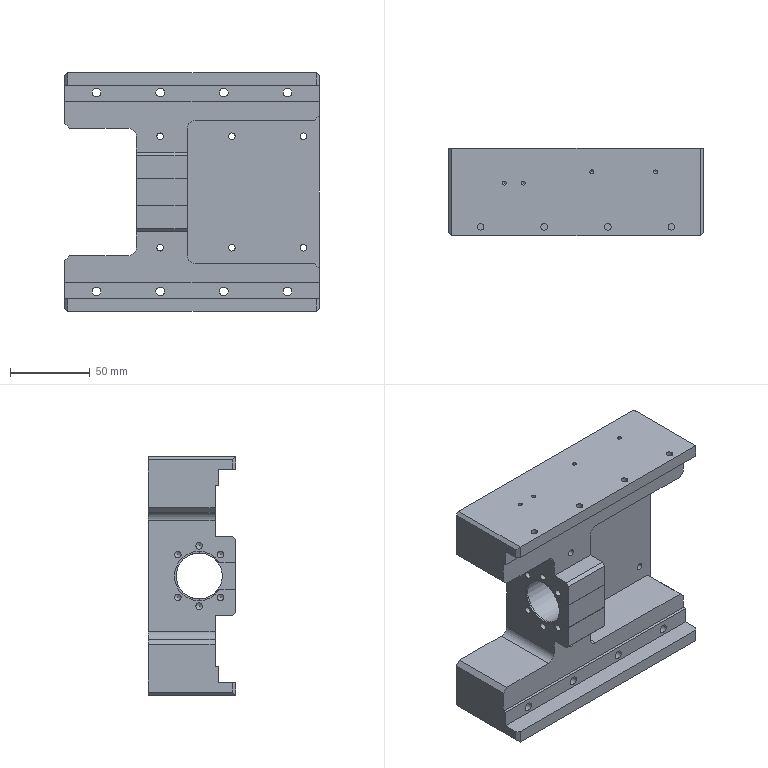Part | 2 solids | 213 faces | box 160 x 55 x 150 mm | volume 1306867 mm3 | plane 101 | cylinder 86 | cone 26 | commonest cylinder face diameters 4.2 x32 10 x24 5.5 x16 2.5 x8 5 x4 29 x2